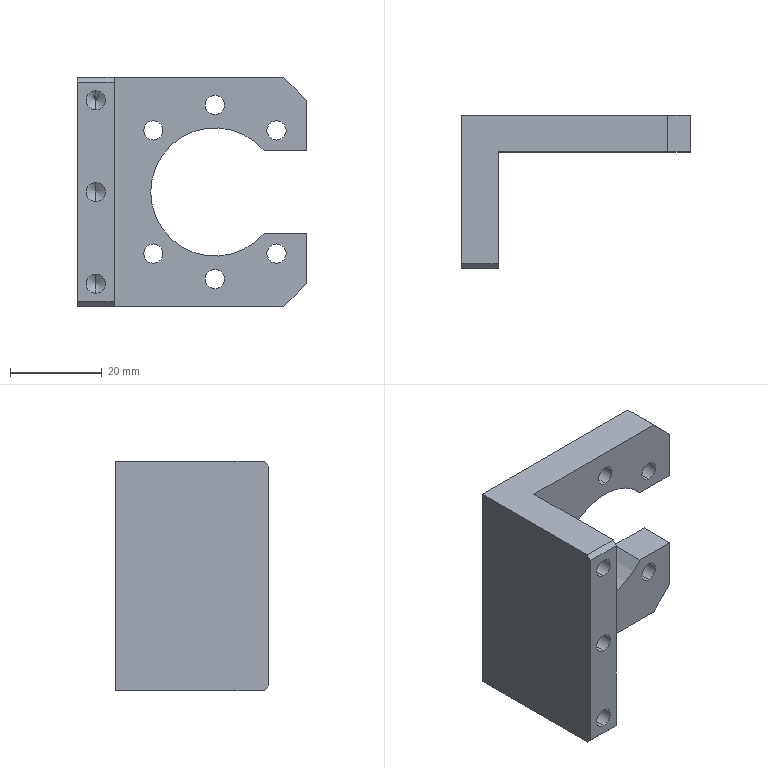Part | STEP file | FBDS-CS-019 | 1 solid | 40 faces | box 50 x 33.5 x 50 mm | volume 22855 mm3 | cylinder 19 | plane 15 | cone 6 | commonest cylinder face diameters 4.2 x18 28 x1
STEP:
#1=CARTESIAN_POINT('',(4.,-21.1,47.1));
#2=VERTEX_POINT('',#1);
#3=CARTESIAN_POINT('',(4.,-21.1,42.9));
#4=VERTEX_POINT('',#3);
#5=CARTESIAN_POINT('',(4.,-21.1,45.));
#6=DIRECTION('',(0.,-1.,0.));
#7=DIRECTION('',(0.,0.,-1.));
#8=AXIS2_PLACEMENT_3D('',#5,#6,#7);
#9=CIRCLE('',#8,2.1);
#10=EDGE_CURVE('',#2,#4,#9,.T.);
#11=ORIENTED_EDGE('',*,*,#10,.F.);
#12=CARTESIAN_POINT('',(4.,-33.5,47.1));
#13=VERTEX_POINT('',#12);
#14=CARTESIAN_POINT('',(4.,-33.5,47.1));
#15=DIRECTION('',(0.,-1.,0.));
#16=VECTOR('',#15,1000.);
#17=LINE('',#14,#16);
#18=EDGE_CURVE('',#2,#13,#17,.T.);
#19=ORIENTED_EDGE('',*,*,#18,.T.);
#20=CARTESIAN_POINT('',(4.,-33.5,42.9));
#21=VERTEX_POINT('',#20);
#22=CARTESIAN_POINT('',(4.,-33.5,45.));
#23=DIRECTION('',(0.,-1.,0.));
#24=DIRECTION('',(0.,0.,-1.));
#25=AXIS2_PLACEMENT_3D('',#22,#23,#24);
#26=CIRCLE('',#25,2.1);
#27=EDGE_CURVE('',#13,#21,#26,.T.);
#28=ORIENTED_EDGE('',*,*,#27,.T.);
#29=CARTESIAN_POINT('',(4.,-33.5,42.9));
#30=DIRECTION('',(0.,-1.,0.));
#31=VECTOR('',#30,1000.);
#32=LINE('',#29,#31);
#33=EDGE_CURVE('',#4,#21,#32,.T.);
#34=ORIENTED_EDGE('',*,*,#33,.F.);
#35=EDGE_LOOP('',(#11,#19,#28,#34));
#36=FACE_OUTER_BOUND('',#35,.T.);
#37=CARTESIAN_POINT('',(4.,-33.5,45.));
#38=DIRECTION('',(0.,-1.,0.));
#39=DIRECTION('',(0.,0.,-1.));
#40=AXIS2_PLACEMENT_3D('',#37,#38,#39);
#41=CYLINDRICAL_SURFACE('',#40,2.1);
#42=ADVANCED_FACE('',(#36),#41,.F.);
#43=CARTESIAN_POINT('',(4.,-19.838,45.));
#44=VERTEX_POINT('',#43);
#45=CARTESIAN_POINT('',(4.,-21.1,42.9));
#46=DIRECTION('',(0.,-0.515,-0.8572));
#47=VECTOR('',#46,1000.);
#48=LINE('',#45,#47);
#49=EDGE_CURVE('',#44,#4,#48,.T.);
#50=ORIENTED_EDGE('',*,*,#49,.F.);
#51=CARTESIAN_POINT('',(4.,-21.1,47.1));
#52=DIRECTION('',(0.,-0.515,0.8572));
#53=VECTOR('',#52,1000.);
#54=LINE('',#51,#53);
#55=EDGE_CURVE('',#44,#2,#54,.T.);
#56=ORIENTED_EDGE('',*,*,#55,.T.);
#57=ORIENTED_EDGE('',*,*,#10,.T.);
#58=EDGE_LOOP('',(#50,#56,#57));
#59=FACE_OUTER_BOUND('',#58,.T.);
#60=CARTESIAN_POINT('',(4.,-21.1,45.));
#61=DIRECTION('',(0.,-1.,0.));
#62=DIRECTION('',(0.,0.,-1.));
#63=AXIS2_PLACEMENT_3D('',#60,#61,#62);
#64=CONICAL_SURFACE('',#63,2.1,1.03);
#65=ADVANCED_FACE('',(#59),#64,.F.);
#66=CARTESIAN_POINT('',(4.,-21.1,27.1));
#67=VERTEX_POINT('',#66);
#68=CARTESIAN_POINT('',(4.,-21.1,22.9));
#69=VERTEX_POINT('',#68);
#70=CARTESIAN_POINT('',(4.,-21.1,25.));
#71=DIRECTION('',(0.,-1.,0.));
#72=DIRECTION('',(0.,0.,-1.));
#73=AXIS2_PLACEMENT_3D('',#70,#71,#72);
#74=CIRCLE('',#73,2.1);
#75=EDGE_CURVE('',#67,#69,#74,.T.);
#76=ORIENTED_EDGE('',*,*,#75,.F.);
#77=CARTESIAN_POINT('',(4.,-33.5,27.1));
#78=VERTEX_POINT('',#77);
#79=CARTESIAN_POINT('',(4.,-33.5,27.1));
#80=DIRECTION('',(0.,-1.,0.));
#81=VECTOR('',#80,1000.);
#82=LINE('',#79,#81);
#83=EDGE_CURVE('',#67,#78,#82,.T.);
#84=ORIENTED_EDGE('',*,*,#83,.T.);
#85=CARTESIAN_POINT('',(4.,-33.5,22.9));
#86=VERTEX_POINT('',#85);
#87=CARTESIAN_POINT('',(4.,-33.5,25.));
#88=DIRECTION('',(0.,-1.,0.));
#89=DIRECTION('',(0.,0.,-1.));
#90=AXIS2_PLACEMENT_3D('',#87,#88,#89);
#91=CIRCLE('',#90,2.1);
#92=EDGE_CURVE('',#78,#86,#91,.T.);
#93=ORIENTED_EDGE('',*,*,#92,.T.);
#94=CARTESIAN_POINT('',(4.,-33.5,22.9));
#95=DIRECTION('',(0.,-1.,0.));
#96=VECTOR('',#95,1000.);
#97=LINE('',#94,#96);
#98=EDGE_CURVE('',#69,#86,#97,.T.);
#99=ORIENTED_EDGE('',*,*,#98,.F.);
#100=EDGE_LOOP('',(#76,#84,#93,#99));
#101=FACE_OUTER_BOUND('',#100,.T.);
#102=CARTESIAN_POINT('',(4.,-33.5,25.));
#103=DIRECTION('',(0.,-1.,0.));
#104=DIRECTION('',(0.,0.,-1.));
#105=AXIS2_PLACEMENT_3D('',#102,#103,#104);
#106=CYLINDRICAL_SURFACE('',#105,2.1);
#107=ADVANCED_FACE('',(#101),#106,.F.);
#108=CARTESIAN_POINT('',(4.,-19.838,25.));
#109=VERTEX_POINT('',#108);
#110=CARTESIAN_POINT('',(4.,-21.1,22.9));
#111=DIRECTION('',(0.,-0.515,-0.8572));
#112=VECTOR('',#111,1000.);
#113=LINE('',#110,#112);
#114=EDGE_CURVE('',#109,#69,#113,.T.);
#115=ORIENTED_EDGE('',*,*,#114,.F.);
#116=CARTESIAN_POINT('',(4.,-21.1,27.1));
#117=DIRECTION('',(0.,-0.515,0.8572));
#118=VECTOR('',#117,1000.);
#119=LINE('',#116,#118);
#120=EDGE_CURVE('',#109,#67,#119,.T.);
#121=ORIENTED_EDGE('',*,*,#120,.T.);
#122=ORIENTED_EDGE('',*,*,#75,.T.);
#123=EDGE_LOOP('',(#115,#121,#122));
#124=FACE_OUTER_BOUND('',#123,.T.);
#125=CARTESIAN_POINT('',(4.,-21.1,25.));
#126=DIRECTION('',(0.,-1.,0.));
#127=DIRECTION('',(0.,0.,-1.));
#128=AXIS2_PLACEMENT_3D('',#125,#126,#127);
#129=CONICAL_SURFACE('',#128,2.1,1.03);
#130=ADVANCED_FACE('',(#124),#129,.F.);
#131=CARTESIAN_POINT('',(4.,-21.1,7.1));
#132=VERTEX_POINT('',#131);
#133=CARTESIAN_POINT('',(4.,-21.1,2.9));
#134=VERTEX_POINT('',#133);
#135=CARTESIAN_POINT('',(4.,-21.1,5.));
#136=DIRECTION('',(0.,-1.,0.));
#137=DIRECTION('',(0.,0.,-1.));
#138=AXIS2_PLACEMENT_3D('',#135,#136,#137);
#139=CIRCLE('',#138,2.1);
#140=EDGE_CURVE('',#132,#134,#139,.T.);
#141=ORIENTED_EDGE('',*,*,#140,.F.);
#142=CARTESIAN_POINT('',(4.,-33.5,7.1));
#143=VERTEX_POINT('',#142);
#144=CARTESIAN_POINT('',(4.,-33.5,7.1));
#145=DIRECTION('',(0.,-1.,0.));
#146=VECTOR('',#145,1000.);
#147=LINE('',#144,#146);
#148=EDGE_CURVE('',#132,#143,#147,.T.);
#149=ORIENTED_EDGE('',*,*,#148,.T.);
#150=CARTESIAN_POINT('',(4.,-33.5,2.9));
#151=VERTEX_POINT('',#150);
#152=CARTESIAN_POINT('',(4.,-33.5,5.));
#153=DIRECTION('',(0.,-1.,0.));
#154=DIRECTION('',(0.,0.,-1.));
#155=AXIS2_PLACEMENT_3D('',#152,#153,#154);
#156=CIRCLE('',#155,2.1);
#157=EDGE_CURVE('',#143,#151,#156,.T.);
#158=ORIENTED_EDGE('',*,*,#157,.T.);
#159=CARTESIAN_POINT('',(4.,-33.5,2.9));
#160=DIRECTION('',(0.,-1.,0.));
#161=VECTOR('',#160,1000.);
#162=LINE('',#159,#161);
#163=EDGE_CURVE('',#134,#151,#162,.T.);
#164=ORIENTED_EDGE('',*,*,#163,.F.);
#165=EDGE_LOOP('',(#141,#149,#158,#164));
#166=FACE_OUTER_BOUND('',#165,.T.);
#167=CARTESIAN_POINT('',(4.,-33.5,5.));
#168=DIRECTION('',(0.,-1.,0.));
#169=DIRECTION('',(0.,0.,-1.));
#170=AXIS2_PLACEMENT_3D('',#167,#168,#169);
#171=CYLINDRICAL_SURFACE('',#170,2.1);
#172=ADVANCED_FACE('',(#166),#171,.F.);
#173=CARTESIAN_POINT('',(4.,-19.838,5.));
#174=VERTEX_POINT('',#173);
#175=CARTESIAN_POINT('',(4.,-21.1,2.9));
#176=DIRECTION('',(0.,-0.515,-0.8572));
#177=VECTOR('',#176,1000.);
#178=LINE('',#175,#177);
#179=EDGE_CURVE('',#174,#134,#178,.T.);
#180=ORIENTED_EDGE('',*,*,#179,.F.);
#181=CARTESIAN_POINT('',(4.,-21.1,7.1));
#182=DIRECTION('',(0.,-0.515,0.8572));
#183=VECTOR('',#182,1000.);
#184=LINE('',#181,#183);
#185=EDGE_CURVE('',#174,#132,#184,.T.);
#186=ORIENTED_EDGE('',*,*,#185,.T.);
#187=ORIENTED_EDGE('',*,*,#140,.T.);
#188=EDGE_LOOP('',(#180,#186,#187));
#189=FACE_OUTER_BOUND('',#188,.T.);
#190=CARTESIAN_POINT('',(4.,-21.1,5.));
#191=DIRECTION('',(0.,-1.,0.));
#192=DIRECTION('',(0.,0.,-1.));
#193=AXIS2_PLACEMENT_3D('',#190,#191,#192);
#194=CONICAL_SURFACE('',#193,2.1,1.03);
#195=ADVANCED_FACE('',(#189),#194,.F.);
#196=CARTESIAN_POINT('',(16.565,0.,13.665));
#197=VERTEX_POINT('',#196);
#198=CARTESIAN_POINT('',(16.565,0.,9.465));
#199=VERTEX_POINT('',#198);
#200=CARTESIAN_POINT('',(16.565,0.,11.565));
#201=DIRECTION('',(0.,-1.,0.));
#202=DIRECTION('',(0.,0.,-1.));
#203=AXIS2_PLACEMENT_3D('',#200,#201,#202);
#204=CIRCLE('',#203,2.1);
#205=EDGE_CURVE('',#197,#199,#204,.T.);
#206=ORIENTED_EDGE('',*,*,#205,.F.);
#207=CARTESIAN_POINT('',(16.565,-8.,13.665));
#208=VERTEX_POINT('',#207);
#209=CARTESIAN_POINT('',(16.565,-8.,13.665));
#210=DIRECTION('',(0.,-1.,0.));
#211=VECTOR('',#210,1000.);
#212=LINE('',#209,#211);
#213=EDGE_CURVE('',#197,#208,#212,.T.);
#214=ORIENTED_EDGE('',*,*,#213,.T.);
#215=CARTESIAN_POINT('',(16.565,-8.,9.465));
#216=VERTEX_POINT('',#215);
#217=CARTESIAN_POINT('',(16.565,-8.,11.565));
#218=DIRECTION('',(0.,-1.,0.));
#219=DIRECTION('',(0.,0.,-1.));
#220=AXIS2_PLACEMENT_3D('',#217,#218,#219);
#221=CIRCLE('',#220,2.1);
#222=EDGE_CURVE('',#208,#216,#221,.T.);
#223=ORIENTED_EDGE('',*,*,#222,.T.);
#224=CARTESIAN_POINT('',(16.565,-8.,9.465));
#225=DIRECTION('',(0.,-1.,0.));
#226=VECTOR('',#225,1000.);
#227=LINE('',#224,#226);
#228=EDGE_CURVE('',#199,#216,#227,.T.);
#229=ORIENTED_EDGE('',*,*,#228,.F.);
#230=EDGE_LOOP('',(#206,#214,#223,#229));
#231=FACE_OUTER_BOUND('',#230,.T.);
#232=CARTESIAN_POINT('',(16.565,-8.,11.565));
#233=DIRECTION('',(0.,-1.,0.));
#234=DIRECTION('',(0.,0.,-1.));
#235=AXIS2_PLACEMENT_3D('',#232,#233,#234);
#236=CYLINDRICAL_SURFACE('',#235,2.1);
#237=ADVANCED_FACE('',(#231),#236,.F.);
#238=CARTESIAN_POINT('',(30.,0.,8.1));
#239=VERTEX_POINT('',#238);
#240=CARTESIAN_POINT('',(30.,0.,3.9));
#241=VERTEX_POINT('',#240);
#242=CARTESIAN_POINT('',(30.,0.,6.));
#243=DIRECTION('',(0.,-1.,0.));
#244=DIRECTION('',(0.,0.,-1.));
#245=AXIS2_PLACEMENT_3D('',#242,#243,#244);
#246=CIRCLE('',#245,2.1);
#247=EDGE_CURVE('',#239,#241,#246,.T.);
#248=ORIENTED_EDGE('',*,*,#247,.F.);
#249=CARTESIAN_POINT('',(30.,-8.,8.1));
#250=VERTEX_POINT('',#249);
#251=CARTESIAN_POINT('',(30.,-8.,8.1));
#252=DIRECTION('',(0.,-1.,0.));
#253=VECTOR('',#252,1000.);
#254=LINE('',#251,#253);
#255=EDGE_CURVE('',#239,#250,#254,.T.);
#256=ORIENTED_EDGE('',*,*,#255,.T.);
#257=CARTESIAN_POINT('',(30.,-8.,3.9));
#258=VERTEX_POINT('',#257);
#259=CARTESIAN_POINT('',(30.,-8.,6.));
#260=DIRECTION('',(0.,-1.,0.));
#261=DIRECTION('',(0.,0.,-1.));
#262=AXIS2_PLACEMENT_3D('',#259,#260,#261);
#263=CIRCLE('',#262,2.1);
#264=EDGE_CURVE('',#250,#258,#263,.T.);
#265=ORIENTED_EDGE('',*,*,#264,.T.);
#266=CARTESIAN_POINT('',(30.,-8.,3.9));
#267=DIRECTION('',(0.,-1.,0.));
#268=VECTOR('',#267,1000.);
#269=LINE('',#266,#268);
#270=EDGE_CURVE('',#241,#258,#269,.T.);
#271=ORIENTED_EDGE('',*,*,#270,.F.);
#272=EDGE_LOOP('',(#248,#256,#265,#271));
#273=FACE_OUTER_BOUND('',#272,.T.);
#274=CARTESIAN_POINT('',(30.,-8.,6.));
#275=DIRECTION('',(0.,-1.,0.));
#276=DIRECTION('',(0.,0.,-1.));
#277=AXIS2_PLACEMENT_3D('',#274,#275,#276);
#278=CYLINDRICAL_SURFACE('',#277,2.1);
#279=ADVANCED_FACE('',(#273),#278,.F.);
#280=CARTESIAN_POINT('',(43.435,0.,13.665));
#281=VERTEX_POINT('',#280);
#282=CARTESIAN_POINT('',(43.435,0.,9.465));
#283=VERTEX_POINT('',#282);
#284=CARTESIAN_POINT('',(43.435,0.,11.565));
#285=DIRECTION('',(0.,-1.,0.));
#286=DIRECTION('',(0.,0.,-1.));
#287=AXIS2_PLACEMENT_3D('',#284,#285,#286);
#288=CIRCLE('',#287,2.1);
#289=EDGE_CURVE('',#281,#283,#288,.T.);
#290=ORIENTED_EDGE('',*,*,#289,.F.);
#291=CARTESIAN_POINT('',(43.435,-8.,13.665));
#292=VERTEX_POINT('',#291);
#293=CARTESIAN_POINT('',(43.435,-8.,13.665));
#294=DIRECTION('',(0.,-1.,0.));
#295=VECTOR('',#294,1000.);
#296=LINE('',#293,#295);
#297=EDGE_CURVE('',#281,#292,#296,.T.);
#298=ORIENTED_EDGE('',*,*,#297,.T.);
#299=CARTESIAN_POINT('',(43.435,-8.,9.465));
#300=VERTEX_POINT('',#299);
#301=CARTESIAN_POINT('',(43.435,-8.,11.565));
#302=DIRECTION('',(0.,-1.,0.));
#303=DIRECTION('',(0.,0.,-1.));
#304=AXIS2_PLACEMENT_3D('',#301,#302,#303);
#305=CIRCLE('',#304,2.1);
#306=EDGE_CURVE('',#292,#300,#305,.T.);
#307=ORIENTED_EDGE('',*,*,#306,.T.);
#308=CARTESIAN_POINT('',(43.435,-8.,9.465));
#309=DIRECTION('',(0.,-1.,0.));
#310=VECTOR('',#309,1000.);
#311=LINE('',#308,#310);
#312=EDGE_CURVE('',#283,#300,#311,.T.);
#313=ORIENTED_EDGE('',*,*,#312,.F.);
#314=EDGE_LOOP('',(#290,#298,#307,#313));
#315=FACE_OUTER_BOUND('',#314,.T.);
#316=CARTESIAN_POINT('',(43.435,-8.,11.565));
#317=DIRECTION('',(0.,-1.,0.));
#318=DIRECTION('',(0.,0.,-1.));
#319=AXIS2_PLACEMENT_3D('',#316,#317,#318);
#320=CYLINDRICAL_SURFACE('',#319,2.1);
#321=ADVANCED_FACE('',(#315),#320,.F.);
#322=CARTESIAN_POINT('',(43.435,0.,40.535));
#323=VERTEX_POINT('',#322);
#324=CARTESIAN_POINT('',(43.435,0.,36.335));
#325=VERTEX_POINT('',#324);
#326=CARTESIAN_POINT('',(43.435,0.,38.435));
#327=DIRECTION('',(0.,-1.,0.));
#328=DIRECTION('',(0.,0.,-1.));
#329=AXIS2_PLACEMENT_3D('',#326,#327,#328);
#330=CIRCLE('',#329,2.1);
#331=EDGE_CURVE('',#323,#325,#330,.T.);
#332=ORIENTED_EDGE('',*,*,#331,.F.);
#333=CARTESIAN_POINT('',(43.435,-8.,40.535));
#334=VERTEX_POINT('',#333);
#335=CARTESIAN_POINT('',(43.435,-8.,40.535));
#336=DIRECTION('',(0.,-1.,0.));
#337=VECTOR('',#336,1000.);
#338=LINE('',#335,#337);
#339=EDGE_CURVE('',#323,#334,#338,.T.);
#340=ORIENTED_EDGE('',*,*,#339,.T.);
#341=CARTESIAN_POINT('',(43.435,-8.,36.335));
#342=VERTEX_POINT('',#341);
#343=CARTESIAN_POINT('',(43.435,-8.,38.435));
#344=DIRECTION('',(0.,-1.,0.));
#345=DIRECTION('',(0.,0.,-1.));
#346=AXIS2_PLACEMENT_3D('',#343,#344,#345);
#347=CIRCLE('',#346,2.1);
#348=EDGE_CURVE('',#334,#342,#347,.T.);
#349=ORIENTED_EDGE('',*,*,#348,.T.);
#350=CARTESIAN_POINT('',(43.435,-8.,36.335));
#351=DIRECTION('',(0.,-1.,0.));
#352=VECTOR('',#351,1000.);
#353=LINE('',#350,#352);
#354=EDGE_CURVE('',#325,#342,#353,.T.);
#355=ORIENTED_EDGE('',*,*,#354,.F.);
#356=EDGE_LOOP('',(#332,#340,#349,#355));
#357=FACE_OUTER_BOUND('',#356,.T.);
#358=CARTESIAN_POINT('',(43.435,-8.,38.435));
#359=DIRECTION('',(0.,-1.,0.));
#360=DIRECTION('',(0.,0.,-1.));
#361=AXIS2_PLACEMENT_3D('',#358,#359,#360);
#362=CYLINDRICAL_SURFACE('',#361,2.1);
#363=ADVANCED_FACE('',(#357),#362,.F.);
#364=CARTESIAN_POINT('',(30.,0.,46.1));
#365=VERTEX_POINT('',#364);
#366=CARTESIAN_POINT('',(30.,0.,41.9));
#367=VERTEX_POINT('',#366);
#368=CARTESIAN_POINT('',(30.,0.,44.));
#369=DIRECTION('',(0.,-1.,0.));
#370=DIRECTION('',(0.,0.,-1.));
#371=AXIS2_PLACEMENT_3D('',#368,#369,#370);
#372=CIRCLE('',#371,2.1);
#373=EDGE_CURVE('',#365,#367,#372,.T.);
#374=ORIENTED_EDGE('',*,*,#373,.F.);
#375=CARTESIAN_POINT('',(30.,-8.,46.1));
#376=VERTEX_POINT('',#375);
#377=CARTESIAN_POINT('',(30.,-8.,46.1));
#378=DIRECTION('',(0.,-1.,0.));
#379=VECTOR('',#378,1000.);
#380=LINE('',#377,#379);
#381=EDGE_CURVE('',#365,#376,#380,.T.);
#382=ORIENTED_EDGE('',*,*,#381,.T.);
#383=CARTESIAN_POINT('',(30.,-8.,41.9));
#384=VERTEX_POINT('',#383);
#385=CARTESIAN_POINT('',(30.,-8.,44.));
#386=DIRECTION('',(0.,-1.,0.));
#387=DIRECTION('',(0.,0.,-1.));
#388=AXIS2_PLACEMENT_3D('',#385,#386,#387);
#389=CIRCLE('',#388,2.1);
#390=EDGE_CURVE('',#376,#384,#389,.T.);
#391=ORIENTED_EDGE('',*,*,#390,.T.);
#392=CARTESIAN_POINT('',(30.,-8.,41.9));
#393=DIRECTION('',(0.,-1.,0.));
#394=VECTOR('',#393,1000.);
#395=LINE('',#392,#394);
#396=EDGE_CURVE('',#367,#384,#395,.T.);
#397=ORIENTED_EDGE('',*,*,#396,.F.);
#398=EDGE_LOOP('',(#374,#382,#391,#397));
#399=FACE_OUTER_BOUND('',#398,.T.);
#400=CARTESIAN_POINT('',(30.,-8.,44.));
#401=DIRECTION('',(0.,-1.,0.));
#402=DIRECTION('',(0.,0.,-1.));
#403=AXIS2_PLACEMENT_3D('',#400,#401,#402);
#404=CYLINDRICAL_SURFACE('',#403,2.1);
#405=ADVANCED_FACE('',(#399),#404,.F.);
#406=CARTESIAN_POINT('',(16.565,0.,40.535));
#407=VERTEX_POINT('',#406);
#408=CARTESIAN_POINT('',(16.565,0.,36.335));
#409=VERTEX_POINT('',#408);
#410=CARTESIAN_POINT('',(16.565,0.,38.435));
#411=DIRECTION('',(0.,-1.,0.));
#412=DIRECTION('',(0.,0.,-1.));
#413=AXIS2_PLACEMENT_3D('',#410,#411,#412);
#414=CIRCLE('',#413,2.1);
#415=EDGE_CURVE('',#407,#409,#414,.T.);
#416=ORIENTED_EDGE('',*,*,#415,.F.);
#417=CARTESIAN_POINT('',(16.565,-8.,40.535));
#418=VERTEX_POINT('',#417);
#419=CARTESIAN_POINT('',(16.565,-8.,40.535));
#420=DIRECTION('',(0.,-1.,0.));
#421=VECTOR('',#420,1000.);
#422=LINE('',#419,#421);
#423=EDGE_CURVE('',#407,#418,#422,.T.);
#424=ORIENTED_EDGE('',*,*,#423,.T.);
#425=CARTESIAN_POINT('',(16.565,-8.,36.335));
#426=VERTEX_POINT('',#425);
#427=CARTESIAN_POINT('',(16.565,-8.,38.435));
#428=DIRECTION('',(0.,-1.,0.));
#429=DIRECTION('',(0.,0.,-1.));
#430=AXIS2_PLACEMENT_3D('',#427,#428,#429);
#431=CIRCLE('',#430,2.1);
#432=EDGE_CURVE('',#418,#426,#431,.T.);
#433=ORIENTED_EDGE('',*,*,#432,.T.);
#434=CARTESIAN_POINT('',(16.565,-8.,36.335));
#435=DIRECTION('',(0.,-1.,0.));
#436=VECTOR('',#435,1000.);
#437=LINE('',#434,#436);
#438=EDGE_CURVE('',#409,#426,#437,.T.);
#439=ORIENTED_EDGE('',*,*,#438,.F.);
#440=EDGE_LOOP('',(#416,#424,#433,#439));
#441=FACE_OUTER_BOUND('',#440,.T.);
#442=CARTESIAN_POINT('',(16.565,-8.,38.435));
#443=DIRECTION('',(0.,-1.,0.));
#444=DIRECTION('',(0.,0.,-1.));
#445=AXIS2_PLACEMENT_3D('',#442,#443,#444);
#446=CYLINDRICAL_SURFACE('',#445,2.1);
#447=ADVANCED_FACE('',(#441),#446,.F.);
#448=CARTESIAN_POINT('',(50.,0.,16.));
#449=VERTEX_POINT('',#448);
#450=CARTESIAN_POINT('',(50.,0.,5.));
#451=VERTEX_POINT('',#450);
#452=CARTESIAN_POINT('',(50.,0.,50.));
#453=DIRECTION('',(0.,0.,-1.));
#454=VECTOR('',#453,1000.);
#455=LINE('',#452,#454);
#456=EDGE_CURVE('',#449,#451,#455,.T.);
#457=ORIENTED_EDGE('',*,*,#456,.F.);
#458=CARTESIAN_POINT('',(50.,-8.,16.));
#459=VERTEX_POINT('',#458);
#460=CARTESIAN_POINT('',(50.,0.,16.));
#461=DIRECTION('',(0.,-1.,0.));
#462=VECTOR('',#461,1000.);
#463=LINE('',#460,#462);
#464=EDGE_CURVE('',#449,#459,#463,.T.);
#465=ORIENTED_EDGE('',*,*,#464,.T.);
#466=CARTESIAN_POINT('',(50.,-8.,5.));
#467=VERTEX_POINT('',#466);
#468=CARTESIAN_POINT('',(50.,-8.,50.));
#469=DIRECTION('',(0.,0.,-1.));
#470=VECTOR('',#469,1000.);
#471=LINE('',#468,#470);
#472=EDGE_CURVE('',#459,#467,#471,.T.);
#473=ORIENTED_EDGE('',*,*,#472,.T.);
#474=CARTESIAN_POINT('',(50.,0.,5.));
#475=DIRECTION('',(0.,1.,0.));
#476=VECTOR('',#475,1000.);
#477=LINE('',#474,#476);
#478=EDGE_CURVE('',#467,#451,#477,.T.);
#479=ORIENTED_EDGE('',*,*,#478,.T.);
#480=EDGE_LOOP('',(#457,#465,#473,#479));
#481=FACE_OUTER_BOUND('',#480,.T.);
#482=CARTESIAN_POINT('',(50.,0.,50.));
#483=DIRECTION('',(-1.,0.,0.));
#484=DIRECTION('',(0.,0.,1.));
#485=AXIS2_PLACEMENT_3D('',#482,#483,#484);
#486=PLANE('',#485);
#487=ADVANCED_FACE('',(#481),#486,.F.);
#488=CARTESIAN_POINT('',(43.435,-8.,11.565));
#489=DIRECTION('',(0.,-1.,0.));
#490=DIRECTION('',(0.,0.,-1.));
#491=AXIS2_PLACEMENT_3D('',#488,#489,#490);
#492=CIRCLE('',#491,2.1);
#493=EDGE_CURVE('',#300,#292,#492,.T.);
#494=ORIENTED_EDGE('',*,*,#493,.F.);
#495=ORIENTED_EDGE('',*,*,#306,.F.);
#496=EDGE_LOOP('',(#494,#495));
#497=FACE_BOUND('',#496,.T.);
#498=ORIENTED_EDGE('',*,*,#472,.F.);
#499=CARTESIAN_POINT('',(40.724,-8.,16.));
#500=VERTEX_POINT('',#499);
#501=CARTESIAN_POINT('',(37.016,-8.,16.));
#502=DIRECTION('',(1.,0.,0.));
#503=VECTOR('',#502,1000.);
#504=LINE('',#501,#503);
#505=EDGE_CURVE('',#500,#459,#504,.T.);
#506=ORIENTED_EDGE('',*,*,#505,.F.);
#507=CARTESIAN_POINT('',(40.724,-8.,34.));
#508=VERTEX_POINT('',#507);
#509=CARTESIAN_POINT('',(30.,-8.,25.));
#510=DIRECTION('',(0.,-1.,0.));
#511=DIRECTION('',(1.,0.,0.));
#512=AXIS2_PLACEMENT_3D('',#509,#510,#511);
#513=CIRCLE('',#512,14.);
#514=EDGE_CURVE('',#508,#500,#513,.T.);
#515=ORIENTED_EDGE('',*,*,#514,.F.);
#516=CARTESIAN_POINT('',(50.,-8.,34.));
#517=VERTEX_POINT('',#516);
#518=CARTESIAN_POINT('',(37.016,-8.,34.));
#519=DIRECTION('',(-1.,0.,0.));
#520=VECTOR('',#519,1000.);
#521=LINE('',#518,#520);
#522=EDGE_CURVE('',#517,#508,#521,.T.);
#523=ORIENTED_EDGE('',*,*,#522,.F.);
#524=CARTESIAN_POINT('',(50.,-8.,45.));
#525=VERTEX_POINT('',#524);
#526=CARTESIAN_POINT('',(50.,-8.,50.));
#527=DIRECTION('',(0.,0.,-1.));
#528=VECTOR('',#527,1000.);
#529=LINE('',#526,#528);
#530=EDGE_CURVE('',#525,#517,#529,.T.);
#531=ORIENTED_EDGE('',*,*,#530,.F.);
#532=CARTESIAN_POINT('',(45.,-8.,50.));
#533=VERTEX_POINT('',#532);
#534=CARTESIAN_POINT('',(45.,-8.,50.));
#535=DIRECTION('',(-0.7071,0.,0.7071));
#536=VECTOR('',#535,1000.);
#537=LINE('',#534,#536);
#538=EDGE_CURVE('',#525,#533,#537,.T.);
#539=ORIENTED_EDGE('',*,*,#538,.T.);
#540=CARTESIAN_POINT('',(8.,-8.,50.));
#541=VERTEX_POINT('',#540);
#542=CARTESIAN_POINT('',(50.,-8.,50.));
#543=DIRECTION('',(1.,0.,0.));
#544=VECTOR('',#543,1000.);
#545=LINE('',#542,#544);
#546=EDGE_CURVE('',#541,#533,#545,.T.);
#547=ORIENTED_EDGE('',*,*,#546,.F.);
#548=CARTESIAN_POINT('',(8.,-8.,0.));
#549=VERTEX_POINT('',#548);
#550=CARTESIAN_POINT('',(8.,-8.,50.));
#551=DIRECTION('',(0.,0.,-1.));
#552=VECTOR('',#551,1000.);
#553=LINE('',#550,#552);
#554=EDGE_CURVE('',#541,#549,#553,.T.);
#555=ORIENTED_EDGE('',*,*,#554,.T.);
#556=CARTESIAN_POINT('',(45.,-8.,0.));
#557=VERTEX_POINT('',#556);
#558=CARTESIAN_POINT('',(50.,-8.,0.));
#559=DIRECTION('',(1.,0.,0.));
#560=VECTOR('',#559,1000.);
#561=LINE('',#558,#560);
#562=EDGE_CURVE('',#549,#557,#561,.T.);
#563=ORIENTED_EDGE('',*,*,#562,.T.);
#564=CARTESIAN_POINT('',(50.,-8.,5.));
#565=DIRECTION('',(0.7071,0.,0.7071));
#566=VECTOR('',#565,1000.);
#567=LINE('',#564,#566);
#568=EDGE_CURVE('',#557,#467,#567,.T.);
#569=ORIENTED_EDGE('',*,*,#568,.T.);
#570=EDGE_LOOP('',(#498,#506,#515,#523,#531,#539,#547,#555,#563,#569));
#571=FACE_OUTER_BOUND('',#570,.T.);
#572=CARTESIAN_POINT('',(16.565,-8.,38.435));
#573=DIRECTION('',(0.,-1.,0.));
#574=DIRECTION('',(0.,0.,-1.));
#575=AXIS2_PLACEMENT_3D('',#572,#573,#574);
#576=CIRCLE('',#575,2.1);
#577=EDGE_CURVE('',#426,#418,#576,.T.);
#578=ORIENTED_EDGE('',*,*,#577,.F.);
#579=ORIENTED_EDGE('',*,*,#432,.F.);
#580=EDGE_LOOP('',(#578,#579));
#581=FACE_BOUND('',#580,.T.);
#582=CARTESIAN_POINT('',(30.,-8.,44.));
#583=DIRECTION('',(0.,-1.,0.));
#584=DIRECTION('',(0.,0.,-1.));
#585=AXIS2_PLACEMENT_3D('',#582,#583,#584);
#586=CIRCLE('',#585,2.1);
#587=EDGE_CURVE('',#384,#376,#586,.T.);
#588=ORIENTED_EDGE('',*,*,#587,.F.);
#589=ORIENTED_EDGE('',*,*,#390,.F.);
#590=EDGE_LOOP('',(#588,#589));
#591=FACE_BOUND('',#590,.T.);
#592=CARTESIAN_POINT('',(43.435,-8.,38.435));
#593=DIRECTION('',(0.,-1.,0.));
#594=DIRECTION('',(0.,0.,-1.));
#595=AXIS2_PLACEMENT_3D('',#592,#593,#594);
#596=CIRCLE('',#595,2.1);
#597=EDGE_CURVE('',#342,#334,#596,.T.);
#598=ORIENTED_EDGE('',*,*,#597,.F.);
#599=ORIENTED_EDGE('',*,*,#348,.F.);
#600=EDGE_LOOP('',(#598,#599));
#601=FACE_BOUND('',#600,.T.);
#602=CARTESIAN_POINT('',(30.,-8.,6.));
#603=DIRECTION('',(0.,-1.,0.));
#604=DIRECTION('',(0.,0.,-1.));
#605=AXIS2_PLACEMENT_3D('',#602,#603,#604);
#606=CIRCLE('',#605,2.1);
#607=EDGE_CURVE('',#258,#250,#606,.T.);
#608=ORIENTED_EDGE('',*,*,#607,.F.);
#609=ORIENTED_EDGE('',*,*,#264,.F.);
#610=EDGE_LOOP('',(#608,#609));
#611=FACE_BOUND('',#610,.T.);
#612=CARTESIAN_POINT('',(16.565,-8.,11.565));
#613=DIRECTION('',(0.,-1.,0.));
#614=DIRECTION('',(0.,0.,-1.));
#615=AXIS2_PLACEMENT_3D('',#612,#613,#614);
#616=CIRCLE('',#615,2.1);
#617=EDGE_CURVE('',#216,#208,#616,.T.);
#618=ORIENTED_EDGE('',*,*,#617,.F.);
#619=ORIENTED_EDGE('',*,*,#222,.F.);
#620=EDGE_LOOP('',(#618,#619));
#621=FACE_BOUND('',#620,.T.);
#622=CARTESIAN_POINT('',(50.,-8.,50.));
#623=DIRECTION('',(0.,1.,0.));
#624=DIRECTION('',(-1.,0.,0.));
#625=AXIS2_PLACEMENT_3D('',#622,#623,#624);
#626=PLANE('',#625);
#627=ADVANCED_FACE('',(#497,#571,#581,#591,#601,#611,#621),#626,.F.);
#628=CARTESIAN_POINT('',(0.,-33.5,49.));
#629=VERTEX_POINT('',#628);
#630=CARTESIAN_POINT('',(0.,-33.5,1.));
#631=VERTEX_POINT('',#630);
#632=CARTESIAN_POINT('',(0.,-33.5,50.));
#633=DIRECTION('',(0.,0.,-1.));
#634=VECTOR('',#633,1000.);
#635=LINE('',#632,#634);
#636=EDGE_CURVE('',#629,#631,#635,.T.);
#637=ORIENTED_EDGE('',*,*,#636,.F.);
#638=CARTESIAN_POINT('',(0.,-32.5,50.));
#639=VERTEX_POINT('',#638);
#640=CARTESIAN_POINT('',(0.,-32.5,50.));
#641=DIRECTION('',(0.,0.7071,0.7071));
#642=VECTOR('',#641,1000.);
#643=LINE('',#640,#642);
#644=EDGE_CURVE('',#629,#639,#643,.T.);
#645=ORIENTED_EDGE('',*,*,#644,.T.);
#646=CARTESIAN_POINT('',(0.,0.,50.));
#647=VERTEX_POINT('',#646);
#648=CARTESIAN_POINT('',(0.,-33.5,50.));
#649=DIRECTION('',(0.,-1.,0.));
#650=VECTOR('',#649,1000.);
#651=LINE('',#648,#650);
#652=EDGE_CURVE('',#647,#639,#651,.T.);
#653=ORIENTED_EDGE('',*,*,#652,.F.);
#654=CARTESIAN_POINT('',(0.,0.,0.));
#655=VERTEX_POINT('',#654);
#656=CARTESIAN_POINT('',(0.,0.,50.));
#657=DIRECTION('',(0.,0.,-1.));
#658=VECTOR('',#657,1000.);
#659=LINE('',#656,#658);
#660=EDGE_CURVE('',#647,#655,#659,.T.);
#661=ORIENTED_EDGE('',*,*,#660,.T.);
#662=CARTESIAN_POINT('',(0.,-32.5,0.));
#663=VERTEX_POINT('',#662);
#664=CARTESIAN_POINT('',(0.,-33.5,0.));
#665=DIRECTION('',(0.,-1.,0.));
#666=VECTOR('',#665,1000.);
#667=LINE('',#664,#666);
#668=EDGE_CURVE('',#655,#663,#667,.T.);
#669=ORIENTED_EDGE('',*,*,#668,.T.);
#670=CARTESIAN_POINT('',(0.,-33.5,1.));
#671=DIRECTION('',(0.,-0.7071,0.7071));
#672=VECTOR('',#671,1000.);
#673=LINE('',#670,#672);
#674=EDGE_CURVE('',#663,#631,#673,.T.);
#675=ORIENTED_EDGE('',*,*,#674,.T.);
#676=EDGE_LOOP('',(#637,#645,#653,#661,#669,#675));
#677=FACE_OUTER_BOUND('',#676,.T.);
#678=CARTESIAN_POINT('',(0.,-33.5,50.));
#679=DIRECTION('',(1.,0.,0.));
#680=DIRECTION('',(0.,0.,-1.));
#681=AXIS2_PLACEMENT_3D('',#678,#679,#680);
#682=PLANE('',#681);
#683=ADVANCED_FACE('',(#677),#682,.F.);
#684=CARTESIAN_POINT('',(4.,-33.5,45.));
#685=DIRECTION('',(0.,-1.,0.));
#686=DIRECTION('',(0.,0.,-1.));
#687=AXIS2_PLACEMENT_3D('',#684,#685,#686);
#688=CIRCLE('',#687,2.1);
#689=EDGE_CURVE('',#21,#13,#688,.T.);
#690=ORIENTED_EDGE('',*,*,#689,.F.);
#691=ORIENTED_EDGE('',*,*,#27,.F.);
#692=EDGE_LOOP('',(#690,#691));
#693=FACE_BOUND('',#692,.T.);
#694=CARTESIAN_POINT('',(4.,-33.5,25.));
#695=DIRECTION('',(0.,-1.,0.));
#696=DIRECTION('',(0.,0.,-1.));
#697=AXIS2_PLACEMENT_3D('',#694,#695,#696);
#698=CIRCLE('',#697,2.1);
#699=EDGE_CURVE('',#86,#78,#698,.T.);
#700=ORIENTED_EDGE('',*,*,#699,.F.);
#701=ORIENTED_EDGE('',*,*,#92,.F.);
#702=EDGE_LOOP('',(#700,#701));
#703=FACE_BOUND('',#702,.T.);
#704=CARTESIAN_POINT('',(4.,-33.5,5.));
#705=DIRECTION('',(0.,-1.,0.));
#706=DIRECTION('',(0.,0.,-1.));
#707=AXIS2_PLACEMENT_3D('',#704,#705,#706);
#708=CIRCLE('',#707,2.1);
#709=EDGE_CURVE('',#151,#143,#708,.T.);
#710=ORIENTED_EDGE('',*,*,#709,.F.);
#711=ORIENTED_EDGE('',*,*,#157,.F.);
#712=EDGE_LOOP('',(#710,#711));
#713=FACE_BOUND('',#712,.T.);
#714=CARTESIAN_POINT('',(8.,-33.5,49.));
#715=VERTEX_POINT('',#714);
#716=CARTESIAN_POINT('',(8.,-33.5,1.));
#717=VERTEX_POINT('',#716);
#718=CARTESIAN_POINT('',(8.,-33.5,50.));
#719=DIRECTION('',(0.,0.,-1.));
#720=VECTOR('',#719,1000.);
#721=LINE('',#718,#720);
#722=EDGE_CURVE('',#715,#717,#721,.T.);
#723=ORIENTED_EDGE('',*,*,#722,.F.);
#724=CARTESIAN_POINT('',(8.,-33.5,49.));
#725=DIRECTION('',(-1.,0.,0.));
#726=VECTOR('',#725,1000.);
#727=LINE('',#724,#726);
#728=EDGE_CURVE('',#715,#629,#727,.T.);
#729=ORIENTED_EDGE('',*,*,#728,.T.);
#730=ORIENTED_EDGE('',*,*,#636,.T.);
#731=CARTESIAN_POINT('',(8.,-33.5,1.));
#732=DIRECTION('',(1.,0.,0.));
#733=VECTOR('',#732,1000.);
#734=LINE('',#731,#733);
#735=EDGE_CURVE('',#631,#717,#734,.T.);
#736=ORIENTED_EDGE('',*,*,#735,.T.);
#737=EDGE_LOOP('',(#723,#729,#730,#736));
#738=FACE_OUTER_BOUND('',#737,.T.);
#739=CARTESIAN_POINT('',(8.,-33.5,50.));
#740=DIRECTION('',(0.,1.,0.));
#741=DIRECTION('',(0.,0.,1.));
#742=AXIS2_PLACEMENT_3D('',#739,#740,#741);
#743=PLANE('',#742);
#744=ADVANCED_FACE('',(#693,#703,#713,#738),#743,.F.);
#745=CARTESIAN_POINT('',(8.,-32.5,50.));
#746=VERTEX_POINT('',#745);
#747=CARTESIAN_POINT('',(8.,-8.,50.));
#748=DIRECTION('',(0.,1.,0.));
#749=VECTOR('',#748,1000.);
#750=LINE('',#747,#749);
#751=EDGE_CURVE('',#746,#541,#750,.T.);
#752=ORIENTED_EDGE('',*,*,#751,.F.);
#753=CARTESIAN_POINT('',(8.,-32.5,50.));
#754=DIRECTION('',(0.,-0.7071,-0.7071));
#755=VECTOR('',#754,1000.);
#756=LINE('',#753,#755);
#757=EDGE_CURVE('',#746,#715,#756,.T.);
#758=ORIENTED_EDGE('',*,*,#757,.T.);
#759=ORIENTED_EDGE('',*,*,#722,.T.);
#760=CARTESIAN_POINT('',(8.,-32.5,0.));
#761=VERTEX_POINT('',#760);
#762=CARTESIAN_POINT('',(8.,-33.5,1.));
#763=DIRECTION('',(0.,0.7071,-0.7071));
#764=VECTOR('',#763,1000.);
#765=LINE('',#762,#764);
#766=EDGE_CURVE('',#717,#761,#765,.T.);
#767=ORIENTED_EDGE('',*,*,#766,.T.);
#768=CARTESIAN_POINT('',(8.,-8.,0.));
#769=DIRECTION('',(0.,1.,0.));
#770=VECTOR('',#769,1000.);
#771=LINE('',#768,#770);
#772=EDGE_CURVE('',#761,#549,#771,.T.);
#773=ORIENTED_EDGE('',*,*,#772,.T.);
#774=ORIENTED_EDGE('',*,*,#554,.F.);
#775=EDGE_LOOP('',(#752,#758,#759,#767,#773,#774));
#776=FACE_OUTER_BOUND('',#775,.T.);
#777=CARTESIAN_POINT('',(8.,-8.,50.));
#778=DIRECTION('',(-1.,0.,0.));
#779=DIRECTION('',(0.,-1.,0.));
#780=AXIS2_PLACEMENT_3D('',#777,#778,#779);
#781=PLANE('',#780);
#782=ADVANCED_FACE('',(#776),#781,.F.);
#783=ORIENTED_EDGE('',*,*,#530,.T.);
#784=CARTESIAN_POINT('',(50.,0.,34.));
#785=VERTEX_POINT('',#784);
#786=CARTESIAN_POINT('',(50.,0.,34.));
#787=DIRECTION('',(0.,1.,0.));
#788=VECTOR('',#787,1000.);
#789=LINE('',#786,#788);
#790=EDGE_CURVE('',#517,#785,#789,.T.);
#791=ORIENTED_EDGE('',*,*,#790,.T.);
#792=CARTESIAN_POINT('',(50.,0.,45.));
#793=VERTEX_POINT('',#792);
#794=CARTESIAN_POINT('',(50.,0.,50.));
#795=DIRECTION('',(0.,0.,-1.));
#796=VECTOR('',#795,1000.);
#797=LINE('',#794,#796);
#798=EDGE_CURVE('',#793,#785,#797,.T.);
#799=ORIENTED_EDGE('',*,*,#798,.F.);
#800=CARTESIAN_POINT('',(50.,0.,45.));
#801=DIRECTION('',(0.,-1.,0.));
#802=VECTOR('',#801,1000.);
#803=LINE('',#800,#802);
#804=EDGE_CURVE('',#793,#525,#803,.T.);
#805=ORIENTED_EDGE('',*,*,#804,.T.);
#806=EDGE_LOOP('',(#783,#791,#799,#805));
#807=FACE_OUTER_BOUND('',#806,.T.);
#808=CARTESIAN_POINT('',(50.,0.,50.));
#809=DIRECTION('',(-1.,0.,0.));
#810=DIRECTION('',(0.,0.,1.));
#811=AXIS2_PLACEMENT_3D('',#808,#809,#810);
#812=PLANE('',#811);
#813=ADVANCED_FACE('',(#807),#812,.F.);
#814=CARTESIAN_POINT('',(16.565,0.,11.565));
#815=DIRECTION('',(0.,-1.,0.));
#816=DIRECTION('',(0.,0.,-1.));
#817=AXIS2_PLACEMENT_3D('',#814,#815,#816);
#818=CIRCLE('',#817,2.1);
#819=EDGE_CURVE('',#199,#197,#818,.T.);
#820=ORIENTED_EDGE('',*,*,#819,.T.);
#821=ORIENTED_EDGE('',*,*,#205,.T.);
#822=EDGE_LOOP('',(#820,#821));
#823=FACE_BOUND('',#822,.T.);
#824=CARTESIAN_POINT('',(30.,0.,6.));
#825=DIRECTION('',(0.,-1.,0.));
#826=DIRECTION('',(0.,0.,-1.));
#827=AXIS2_PLACEMENT_3D('',#824,#825,#826);
#828=CIRCLE('',#827,2.1);
#829=EDGE_CURVE('',#241,#239,#828,.T.);
#830=ORIENTED_EDGE('',*,*,#829,.T.);
#831=ORIENTED_EDGE('',*,*,#247,.T.);
#832=EDGE_LOOP('',(#830,#831));
#833=FACE_BOUND('',#832,.T.);
#834=CARTESIAN_POINT('',(43.435,0.,11.565));
#835=DIRECTION('',(0.,-1.,0.));
#836=DIRECTION('',(0.,0.,-1.));
#837=AXIS2_PLACEMENT_3D('',#834,#835,#836);
#838=CIRCLE('',#837,2.1);
#839=EDGE_CURVE('',#283,#281,#838,.T.);
#840=ORIENTED_EDGE('',*,*,#839,.T.);
#841=ORIENTED_EDGE('',*,*,#289,.T.);
#842=EDGE_LOOP('',(#840,#841));
#843=FACE_BOUND('',#842,.T.);
#844=CARTESIAN_POINT('',(43.435,0.,38.435));
#845=DIRECTION('',(0.,-1.,0.));
#846=DIRECTION('',(0.,0.,-1.));
#847=AXIS2_PLACEMENT_3D('',#844,#845,#846);
#848=CIRCLE('',#847,2.1);
#849=EDGE_CURVE('',#325,#323,#848,.T.);
#850=ORIENTED_EDGE('',*,*,#849,.T.);
#851=ORIENTED_EDGE('',*,*,#331,.T.);
#852=EDGE_LOOP('',(#850,#851));
#853=FACE_BOUND('',#852,.T.);
#854=CARTESIAN_POINT('',(30.,0.,44.));
#855=DIRECTION('',(0.,-1.,0.));
#856=DIRECTION('',(0.,0.,-1.));
#857=AXIS2_PLACEMENT_3D('',#854,#855,#856);
#858=CIRCLE('',#857,2.1);
#859=EDGE_CURVE('',#367,#365,#858,.T.);
#860=ORIENTED_EDGE('',*,*,#859,.T.);
#861=ORIENTED_EDGE('',*,*,#373,.T.);
#862=EDGE_LOOP('',(#860,#861));
#863=FACE_BOUND('',#862,.T.);
#864=CARTESIAN_POINT('',(16.565,0.,38.435));
#865=DIRECTION('',(0.,-1.,0.));
#866=DIRECTION('',(0.,0.,-1.));
#867=AXIS2_PLACEMENT_3D('',#864,#865,#866);
#868=CIRCLE('',#867,2.1);
#869=EDGE_CURVE('',#409,#407,#868,.T.);
#870=ORIENTED_EDGE('',*,*,#869,.T.);
#871=ORIENTED_EDGE('',*,*,#415,.T.);
#872=EDGE_LOOP('',(#870,#871));
#873=FACE_BOUND('',#872,.T.);
#874=CARTESIAN_POINT('',(40.724,0.,34.));
#875=VERTEX_POINT('',#874);
#876=CARTESIAN_POINT('',(40.724,0.,16.));
#877=VERTEX_POINT('',#876);
#878=CARTESIAN_POINT('',(30.,0.,25.));
#879=DIRECTION('',(0.,-1.,0.));
#880=DIRECTION('',(0.,0.,-1.));
#881=AXIS2_PLACEMENT_3D('',#878,#879,#880);
#882=CIRCLE('',#881,14.);
#883=EDGE_CURVE('',#875,#877,#882,.T.);
#884=ORIENTED_EDGE('',*,*,#883,.T.);
#885=CARTESIAN_POINT('',(0.,0.,16.));
#886=DIRECTION('',(1.,0.,0.));
#887=VECTOR('',#886,1000.);
#888=LINE('',#885,#887);
#889=EDGE_CURVE('',#877,#449,#888,.T.);
#890=ORIENTED_EDGE('',*,*,#889,.T.);
#891=ORIENTED_EDGE('',*,*,#456,.T.);
#892=CARTESIAN_POINT('',(45.,0.,0.));
#893=VERTEX_POINT('',#892);
#894=CARTESIAN_POINT('',(50.,0.,5.));
#895=DIRECTION('',(-0.7071,0.,-0.7071));
#896=VECTOR('',#895,1000.);
#897=LINE('',#894,#896);
#898=EDGE_CURVE('',#451,#893,#897,.T.);
#899=ORIENTED_EDGE('',*,*,#898,.T.);
#900=CARTESIAN_POINT('',(0.,0.,0.));
#901=DIRECTION('',(-1.,0.,0.));
#902=VECTOR('',#901,1000.);
#903=LINE('',#900,#902);
#904=EDGE_CURVE('',#893,#655,#903,.T.);
#905=ORIENTED_EDGE('',*,*,#904,.T.);
#906=ORIENTED_EDGE('',*,*,#660,.F.);
#907=CARTESIAN_POINT('',(45.,0.,50.));
#908=VERTEX_POINT('',#907);
#909=CARTESIAN_POINT('',(0.,0.,50.));
#910=DIRECTION('',(-1.,0.,0.));
#911=VECTOR('',#910,1000.);
#912=LINE('',#909,#911);
#913=EDGE_CURVE('',#908,#647,#912,.T.);
#914=ORIENTED_EDGE('',*,*,#913,.F.);
#915=CARTESIAN_POINT('',(45.,0.,50.));
#916=DIRECTION('',(0.7071,0.,-0.7071));
#917=VECTOR('',#916,1000.);
#918=LINE('',#915,#917);
#919=EDGE_CURVE('',#908,#793,#918,.T.);
#920=ORIENTED_EDGE('',*,*,#919,.T.);
#921=ORIENTED_EDGE('',*,*,#798,.T.);
#922=CARTESIAN_POINT('',(0.,0.,34.));
#923=DIRECTION('',(-1.,0.,0.));
#924=VECTOR('',#923,1000.);
#925=LINE('',#922,#924);
#926=EDGE_CURVE('',#785,#875,#925,.T.);
#927=ORIENTED_EDGE('',*,*,#926,.T.);
#928=EDGE_LOOP('',(#884,#890,#891,#899,#905,#906,#914,#920,#921,#927));
#929=FACE_OUTER_BOUND('',#928,.T.);
#930=CARTESIAN_POINT('',(0.,0.,50.));
#931=DIRECTION('',(0.,-1.,0.));
#932=DIRECTION('',(0.,0.,-1.));
#933=AXIS2_PLACEMENT_3D('',#930,#931,#932);
#934=PLANE('',#933);
#935=ADVANCED_FACE('',(#823,#833,#843,#853,#863,#873,#929),#934,.F.);
#936=ORIENTED_EDGE('',*,*,#652,.T.);
#937=CARTESIAN_POINT('',(0.,-32.5,50.));
#938=DIRECTION('',(1.,0.,0.));
#939=VECTOR('',#938,1000.);
#940=LINE('',#937,#939);
#941=EDGE_CURVE('',#639,#746,#940,.T.);
#942=ORIENTED_EDGE('',*,*,#941,.T.);
#943=ORIENTED_EDGE('',*,*,#751,.T.);
#944=ORIENTED_EDGE('',*,*,#546,.T.);
#945=CARTESIAN_POINT('',(45.,0.,50.));
#946=DIRECTION('',(0.,1.,0.));
#947=VECTOR('',#946,1000.);
#948=LINE('',#945,#947);
#949=EDGE_CURVE('',#533,#908,#948,.T.);
#950=ORIENTED_EDGE('',*,*,#949,.T.);
#951=ORIENTED_EDGE('',*,*,#913,.T.);
#952=EDGE_LOOP('',(#936,#942,#943,#944,#950,#951));
#953=FACE_OUTER_BOUND('',#952,.T.);
#954=CARTESIAN_POINT('',(0.,0.,50.));
#955=DIRECTION('',(0.,0.,-1.));
#956=DIRECTION('',(-1.,0.,0.));
#957=AXIS2_PLACEMENT_3D('',#954,#955,#956);
#958=PLANE('',#957);
#959=ADVANCED_FACE('',(#953),#958,.F.);
#960=ORIENTED_EDGE('',*,*,#772,.F.);
#961=CARTESIAN_POINT('',(0.,-32.5,0.));
#962=DIRECTION('',(-1.,0.,0.));
#963=VECTOR('',#962,1000.);
#964=LINE('',#961,#963);
#965=EDGE_CURVE('',#761,#663,#964,.T.);
#966=ORIENTED_EDGE('',*,*,#965,.T.);
#967=ORIENTED_EDGE('',*,*,#668,.F.);
#968=ORIENTED_EDGE('',*,*,#904,.F.);
#969=CARTESIAN_POINT('',(45.,-8.,0.));
#970=DIRECTION('',(0.,-1.,0.));
#971=VECTOR('',#970,1000.);
#972=LINE('',#969,#971);
#973=EDGE_CURVE('',#893,#557,#972,.T.);
#974=ORIENTED_EDGE('',*,*,#973,.T.);
#975=ORIENTED_EDGE('',*,*,#562,.F.);
#976=EDGE_LOOP('',(#960,#966,#967,#968,#974,#975));
#977=FACE_OUTER_BOUND('',#976,.T.);
#978=CARTESIAN_POINT('',(0.,0.,0.));
#979=DIRECTION('',(0.,0.,-1.));
#980=DIRECTION('',(-1.,0.,0.));
#981=AXIS2_PLACEMENT_3D('',#978,#979,#980);
#982=PLANE('',#981);
#983=ADVANCED_FACE('',(#977),#982,.T.);
#984=ORIENTED_EDGE('',*,*,#514,.T.);
#985=CARTESIAN_POINT('',(40.724,2.,16.));
#986=DIRECTION('',(0.,1.,0.));
#987=VECTOR('',#986,1000.);
#988=LINE('',#985,#987);
#989=EDGE_CURVE('',#500,#877,#988,.T.);
#990=ORIENTED_EDGE('',*,*,#989,.T.);
#991=ORIENTED_EDGE('',*,*,#883,.F.);
#992=CARTESIAN_POINT('',(40.724,2.,34.));
#993=DIRECTION('',(0.,-1.,0.));
#994=VECTOR('',#993,1000.);
#995=LINE('',#992,#994);
#996=EDGE_CURVE('',#875,#508,#995,.T.);
#997=ORIENTED_EDGE('',*,*,#996,.T.);
#998=EDGE_LOOP('',(#984,#990,#991,#997));
#999=FACE_OUTER_BOUND('',#998,.T.);
#1000=CARTESIAN_POINT('',(30.,2.,25.));
#1001=DIRECTION('',(0.,-1.,0.));
#1002=DIRECTION('',(1.,0.,0.));
#1003=AXIS2_PLACEMENT_3D('',#1000,#1001,#1002);
#1004=CYLINDRICAL_SURFACE('',#1003,14.);
#1005=ADVANCED_FACE('',(#999),#1004,.F.);
#1006=ORIENTED_EDGE('',*,*,#538,.F.);
#1007=ORIENTED_EDGE('',*,*,#804,.F.);
#1008=ORIENTED_EDGE('',*,*,#919,.F.);
#1009=ORIENTED_EDGE('',*,*,#949,.F.);
#1010=EDGE_LOOP('',(#1006,#1007,#1008,#1009));
#1011=FACE_OUTER_BOUND('',#1010,.T.);
#1012=CARTESIAN_POINT('',(45.,0.,50.));
#1013=DIRECTION('',(-0.7071,0.,-0.7071));
#1014=DIRECTION('',(0.,1.,0.));
#1015=AXIS2_PLACEMENT_3D('',#1012,#1013,#1014);
#1016=PLANE('',#1015);
#1017=ADVANCED_FACE('',(#1011),#1016,.F.);
#1018=ORIENTED_EDGE('',*,*,#568,.F.);
#1019=ORIENTED_EDGE('',*,*,#973,.F.);
#1020=ORIENTED_EDGE('',*,*,#898,.F.);
#1021=ORIENTED_EDGE('',*,*,#478,.F.);
#1022=EDGE_LOOP('',(#1018,#1019,#1020,#1021));
#1023=FACE_OUTER_BOUND('',#1022,.T.);
#1024=CARTESIAN_POINT('',(50.,0.,5.));
#1025=DIRECTION('',(0.7071,0.,-0.7071));
#1026=DIRECTION('',(0.,-1.,0.));
#1027=AXIS2_PLACEMENT_3D('',#1024,#1025,#1026);
#1028=PLANE('',#1027);
#1029=ADVANCED_FACE('',(#1023),#1028,.T.);
#1030=ORIENTED_EDGE('',*,*,#423,.F.);
#1031=ORIENTED_EDGE('',*,*,#869,.F.);
#1032=ORIENTED_EDGE('',*,*,#438,.T.);
#1033=ORIENTED_EDGE('',*,*,#577,.T.);
#1034=EDGE_LOOP('',(#1030,#1031,#1032,#1033));
#1035=FACE_OUTER_BOUND('',#1034,.T.);
#1036=CARTESIAN_POINT('',(16.565,-8.,38.435));
#1037=DIRECTION('',(0.,-1.,0.));
#1038=DIRECTION('',(0.,0.,-1.));
#1039=AXIS2_PLACEMENT_3D('',#1036,#1037,#1038);
#1040=CYLINDRICAL_SURFACE('',#1039,2.1);
#1041=ADVANCED_FACE('',(#1035),#1040,.F.);
#1042=ORIENTED_EDGE('',*,*,#381,.F.);
#1043=ORIENTED_EDGE('',*,*,#859,.F.);
#1044=ORIENTED_EDGE('',*,*,#396,.T.);
#1045=ORIENTED_EDGE('',*,*,#587,.T.);
#1046=EDGE_LOOP('',(#1042,#1043,#1044,#1045));
#1047=FACE_OUTER_BOUND('',#1046,.T.);
#1048=CARTESIAN_POINT('',(30.,-8.,44.));
#1049=DIRECTION('',(0.,-1.,0.));
#1050=DIRECTION('',(0.,0.,-1.));
#1051=AXIS2_PLACEMENT_3D('',#1048,#1049,#1050);
#1052=CYLINDRICAL_SURFACE('',#1051,2.1);
#1053=ADVANCED_FACE('',(#1047),#1052,.F.);
#1054=ORIENTED_EDGE('',*,*,#339,.F.);
#1055=ORIENTED_EDGE('',*,*,#849,.F.);
#1056=ORIENTED_EDGE('',*,*,#354,.T.);
#1057=ORIENTED_EDGE('',*,*,#597,.T.);
#1058=EDGE_LOOP('',(#1054,#1055,#1056,#1057));
#1059=FACE_OUTER_BOUND('',#1058,.T.);
#1060=CARTESIAN_POINT('',(43.435,-8.,38.435));
#1061=DIRECTION('',(0.,-1.,0.));
#1062=DIRECTION('',(0.,0.,-1.));
#1063=AXIS2_PLACEMENT_3D('',#1060,#1061,#1062);
#1064=CYLINDRICAL_SURFACE('',#1063,2.1);
#1065=ADVANCED_FACE('',(#1059),#1064,.F.);
#1066=ORIENTED_EDGE('',*,*,#297,.F.);
#1067=ORIENTED_EDGE('',*,*,#839,.F.);
#1068=ORIENTED_EDGE('',*,*,#312,.T.);
#1069=ORIENTED_EDGE('',*,*,#493,.T.);
#1070=EDGE_LOOP('',(#1066,#1067,#1068,#1069));
#1071=FACE_OUTER_BOUND('',#1070,.T.);
#1072=CARTESIAN_POINT('',(43.435,-8.,11.565));
#1073=DIRECTION('',(0.,-1.,0.));
#1074=DIRECTION('',(0.,0.,-1.));
#1075=AXIS2_PLACEMENT_3D('',#1072,#1073,#1074);
#1076=CYLINDRICAL_SURFACE('',#1075,2.1);
#1077=ADVANCED_FACE('',(#1071),#1076,.F.);
#1078=ORIENTED_EDGE('',*,*,#255,.F.);
#1079=ORIENTED_EDGE('',*,*,#829,.F.);
#1080=ORIENTED_EDGE('',*,*,#270,.T.);
#1081=ORIENTED_EDGE('',*,*,#607,.T.);
#1082=EDGE_LOOP('',(#1078,#1079,#1080,#1081));
#1083=FACE_OUTER_BOUND('',#1082,.T.);
#1084=CARTESIAN_POINT('',(30.,-8.,6.));
#1085=DIRECTION('',(0.,-1.,0.));
#1086=DIRECTION('',(0.,0.,-1.));
#1087=AXIS2_PLACEMENT_3D('',#1084,#1085,#1086);
#1088=CYLINDRICAL_SURFACE('',#1087,2.1);
#1089=ADVANCED_FACE('',(#1083),#1088,.F.);
#1090=ORIENTED_EDGE('',*,*,#213,.F.);
#1091=ORIENTED_EDGE('',*,*,#819,.F.);
#1092=ORIENTED_EDGE('',*,*,#228,.T.);
#1093=ORIENTED_EDGE('',*,*,#617,.T.);
#1094=EDGE_LOOP('',(#1090,#1091,#1092,#1093));
#1095=FACE_OUTER_BOUND('',#1094,.T.);
#1096=CARTESIAN_POINT('',(16.565,-8.,11.565));
#1097=DIRECTION('',(0.,-1.,0.));
#1098=DIRECTION('',(0.,0.,-1.));
#1099=AXIS2_PLACEMENT_3D('',#1096,#1097,#1098);
#1100=CYLINDRICAL_SURFACE('',#1099,2.1);
#1101=ADVANCED_FACE('',(#1095),#1100,.F.);
#1102=ORIENTED_EDGE('',*,*,#522,.T.);
#1103=ORIENTED_EDGE('',*,*,#996,.F.);
#1104=ORIENTED_EDGE('',*,*,#926,.F.);
#1105=ORIENTED_EDGE('',*,*,#790,.F.);
#1106=EDGE_LOOP('',(#1102,#1103,#1104,#1105));
#1107=FACE_OUTER_BOUND('',#1106,.T.);
#1108=CARTESIAN_POINT('',(37.016,2.,34.));
#1109=DIRECTION('',(0.,0.,1.));
#1110=DIRECTION('',(1.,0.,0.));
#1111=AXIS2_PLACEMENT_3D('',#1108,#1109,#1110);
#1112=PLANE('',#1111);
#1113=ADVANCED_FACE('',(#1107),#1112,.F.);
#1114=ORIENTED_EDGE('',*,*,#889,.F.);
#1115=ORIENTED_EDGE('',*,*,#989,.F.);
#1116=ORIENTED_EDGE('',*,*,#505,.T.);
#1117=ORIENTED_EDGE('',*,*,#464,.F.);
#1118=EDGE_LOOP('',(#1114,#1115,#1116,#1117));
#1119=FACE_OUTER_BOUND('',#1118,.T.);
#1120=CARTESIAN_POINT('',(37.016,2.,16.));
#1121=DIRECTION('',(0.,0.,-1.));
#1122=DIRECTION('',(-1.,0.,0.));
#1123=AXIS2_PLACEMENT_3D('',#1120,#1121,#1122);
#1124=PLANE('',#1123);
#1125=ADVANCED_FACE('',(#1119),#1124,.F.);
#1126=ORIENTED_EDGE('',*,*,#185,.F.);
#1127=ORIENTED_EDGE('',*,*,#179,.T.);
#1128=CARTESIAN_POINT('',(4.,-21.1,5.));
#1129=DIRECTION('',(0.,-1.,0.));
#1130=DIRECTION('',(0.,0.,-1.));
#1131=AXIS2_PLACEMENT_3D('',#1128,#1129,#1130);
#1132=CIRCLE('',#1131,2.1);
#1133=EDGE_CURVE('',#134,#132,#1132,.T.);
#1134=ORIENTED_EDGE('',*,*,#1133,.T.);
#1135=EDGE_LOOP('',(#1126,#1127,#1134));
#1136=FACE_OUTER_BOUND('',#1135,.T.);
#1137=CARTESIAN_POINT('',(4.,-21.1,5.));
#1138=DIRECTION('',(0.,-1.,0.));
#1139=DIRECTION('',(0.,0.,-1.));
#1140=AXIS2_PLACEMENT_3D('',#1137,#1138,#1139);
#1141=CONICAL_SURFACE('',#1140,2.1,1.03);
#1142=ADVANCED_FACE('',(#1136),#1141,.F.);
#1143=ORIENTED_EDGE('',*,*,#148,.F.);
#1144=ORIENTED_EDGE('',*,*,#1133,.F.);
#1145=ORIENTED_EDGE('',*,*,#163,.T.);
#1146=ORIENTED_EDGE('',*,*,#709,.T.);
#1147=EDGE_LOOP('',(#1143,#1144,#1145,#1146));
#1148=FACE_OUTER_BOUND('',#1147,.T.);
#1149=CARTESIAN_POINT('',(4.,-33.5,5.));
#1150=DIRECTION('',(0.,-1.,0.));
#1151=DIRECTION('',(0.,0.,-1.));
#1152=AXIS2_PLACEMENT_3D('',#1149,#1150,#1151);
#1153=CYLINDRICAL_SURFACE('',#1152,2.1);
#1154=ADVANCED_FACE('',(#1148),#1153,.F.);
#1155=ORIENTED_EDGE('',*,*,#120,.F.);
#1156=ORIENTED_EDGE('',*,*,#114,.T.);
#1157=CARTESIAN_POINT('',(4.,-21.1,25.));
#1158=DIRECTION('',(0.,-1.,0.));
#1159=DIRECTION('',(0.,0.,-1.));
#1160=AXIS2_PLACEMENT_3D('',#1157,#1158,#1159);
#1161=CIRCLE('',#1160,2.1);
#1162=EDGE_CURVE('',#69,#67,#1161,.T.);
#1163=ORIENTED_EDGE('',*,*,#1162,.T.);
#1164=EDGE_LOOP('',(#1155,#1156,#1163));
#1165=FACE_OUTER_BOUND('',#1164,.T.);
#1166=CARTESIAN_POINT('',(4.,-21.1,25.));
#1167=DIRECTION('',(0.,-1.,0.));
#1168=DIRECTION('',(0.,0.,-1.));
#1169=AXIS2_PLACEMENT_3D('',#1166,#1167,#1168);
#1170=CONICAL_SURFACE('',#1169,2.1,1.03);
#1171=ADVANCED_FACE('',(#1165),#1170,.F.);
#1172=ORIENTED_EDGE('',*,*,#83,.F.);
#1173=ORIENTED_EDGE('',*,*,#1162,.F.);
#1174=ORIENTED_EDGE('',*,*,#98,.T.);
#1175=ORIENTED_EDGE('',*,*,#699,.T.);
#1176=EDGE_LOOP('',(#1172,#1173,#1174,#1175));
#1177=FACE_OUTER_BOUND('',#1176,.T.);
#1178=CARTESIAN_POINT('',(4.,-33.5,25.));
#1179=DIRECTION('',(0.,-1.,0.));
#1180=DIRECTION('',(0.,0.,-1.));
#1181=AXIS2_PLACEMENT_3D('',#1178,#1179,#1180);
#1182=CYLINDRICAL_SURFACE('',#1181,2.1);
#1183=ADVANCED_FACE('',(#1177),#1182,.F.);
#1184=ORIENTED_EDGE('',*,*,#55,.F.);
#1185=ORIENTED_EDGE('',*,*,#49,.T.);
#1186=CARTESIAN_POINT('',(4.,-21.1,45.));
#1187=DIRECTION('',(0.,-1.,0.));
#1188=DIRECTION('',(0.,0.,-1.));
#1189=AXIS2_PLACEMENT_3D('',#1186,#1187,#1188);
#1190=CIRCLE('',#1189,2.1);
#1191=EDGE_CURVE('',#4,#2,#1190,.T.);
#1192=ORIENTED_EDGE('',*,*,#1191,.T.);
#1193=EDGE_LOOP('',(#1184,#1185,#1192));
#1194=FACE_OUTER_BOUND('',#1193,.T.);
#1195=CARTESIAN_POINT('',(4.,-21.1,45.));
#1196=DIRECTION('',(0.,-1.,0.));
#1197=DIRECTION('',(0.,0.,-1.));
#1198=AXIS2_PLACEMENT_3D('',#1195,#1196,#1197);
#1199=CONICAL_SURFACE('',#1198,2.1,1.03);
#1200=ADVANCED_FACE('',(#1194),#1199,.F.);
#1201=ORIENTED_EDGE('',*,*,#18,.F.);
#1202=ORIENTED_EDGE('',*,*,#1191,.F.);
#1203=ORIENTED_EDGE('',*,*,#33,.T.);
#1204=ORIENTED_EDGE('',*,*,#689,.T.);
#1205=EDGE_LOOP('',(#1201,#1202,#1203,#1204));
#1206=FACE_OUTER_BOUND('',#1205,.T.);
#1207=CARTESIAN_POINT('',(4.,-33.5,45.));
#1208=DIRECTION('',(0.,-1.,0.));
#1209=DIRECTION('',(0.,0.,-1.));
#1210=AXIS2_PLACEMENT_3D('',#1207,#1208,#1209);
#1211=CYLINDRICAL_SURFACE('',#1210,2.1);
#1212=ADVANCED_FACE('',(#1206),#1211,.F.);
#1213=ORIENTED_EDGE('',*,*,#644,.F.);
#1214=ORIENTED_EDGE('',*,*,#728,.F.);
#1215=ORIENTED_EDGE('',*,*,#757,.F.);
#1216=ORIENTED_EDGE('',*,*,#941,.F.);
#1217=EDGE_LOOP('',(#1213,#1214,#1215,#1216));
#1218=FACE_OUTER_BOUND('',#1217,.T.);
#1219=CARTESIAN_POINT('',(0.,-32.5,50.));
#1220=DIRECTION('',(0.,0.7071,-0.7071));
#1221=DIRECTION('',(1.,0.,0.));
#1222=AXIS2_PLACEMENT_3D('',#1219,#1220,#1221);
#1223=PLANE('',#1222);
#1224=ADVANCED_FACE('',(#1218),#1223,.F.);
#1225=ORIENTED_EDGE('',*,*,#674,.F.);
#1226=ORIENTED_EDGE('',*,*,#965,.F.);
#1227=ORIENTED_EDGE('',*,*,#766,.F.);
#1228=ORIENTED_EDGE('',*,*,#735,.F.);
#1229=EDGE_LOOP('',(#1225,#1226,#1227,#1228));
#1230=FACE_OUTER_BOUND('',#1229,.T.);
#1231=CARTESIAN_POINT('',(8.,-33.5,1.));
#1232=DIRECTION('',(0.,-0.7071,-0.7071));
#1233=DIRECTION('',(-1.,0.,0.));
#1234=AXIS2_PLACEMENT_3D('',#1231,#1232,#1233);
#1235=PLANE('',#1234);
#1236=ADVANCED_FACE('',(#1230),#1235,.T.);
#1237=CLOSED_SHELL('',(#42,#65,#107,#130,#172,#195,#237,#279,#321,#363,#405,#447,#487,#627,#683,#744,#782,#813,#935,#959,#983,#1005,#1017,#1029,#1041,#1053,#1065,#1077,#1089,#1101,#1113,#1125,#1142,#1154,#1171,#1183,#1200,#1212,#1224,#1236));
#1238=MANIFOLD_SOLID_BREP('',#1237);
#1239=CARTESIAN_POINT('',(0.,0.,0.));
#1240=DIRECTION('',(0.,0.,1.));
#1241=DIRECTION('',(1.,0.,0.));
#1242=AXIS2_PLACEMENT_3D('',#1239,#1240,#1241);
#1243=(LENGTH_UNIT()NAMED_UNIT(*)SI_UNIT(.MILLI.,.METRE.));
#1244=UNCERTAINTY_MEASURE_WITH_UNIT(LENGTH_MEASURE(0.00001),#1243,'','');
#1245=(NAMED_UNIT(*)PLANE_ANGLE_UNIT()SI_UNIT($,.RADIAN.));
#1246=(NAMED_UNIT(*)SI_UNIT($,.STERADIAN.)SOLID_ANGLE_UNIT());
#1247=(GEOMETRIC_REPRESENTATION_CONTEXT(3)GLOBAL_UNCERTAINTY_ASSIGNED_CONTEXT((#1244))GLOBAL_UNIT_ASSIGNED_CONTEXT((#1243,#1245,#1246))REPRESENTATION_CONTEXT('',''));
#1248=ADVANCED_BREP_SHAPE_REPRESENTATION('',(#1238,#1242),#1247);